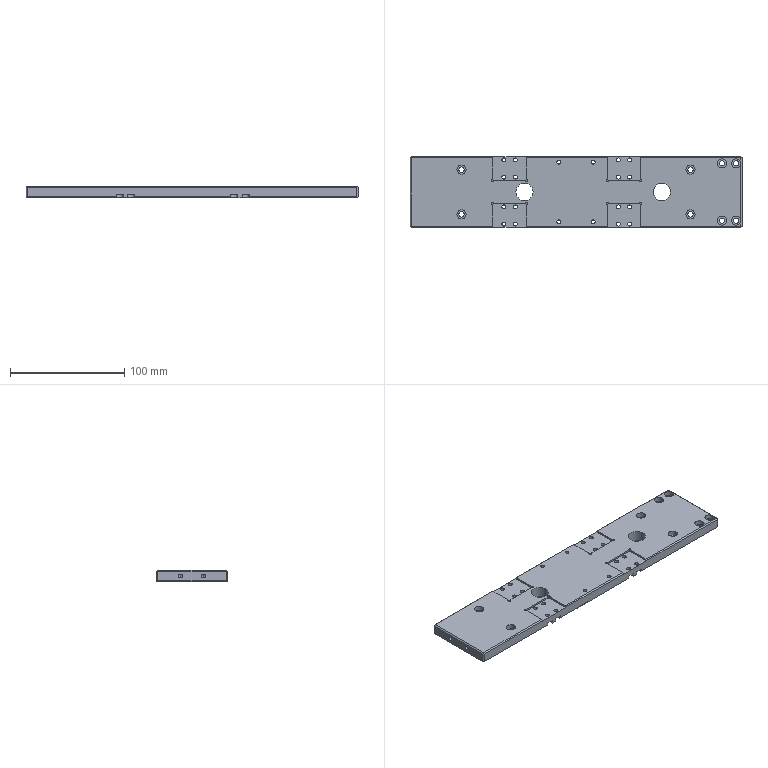Part | STEP file | 01-03 loading sliding base plate | 1 solid | 214 faces | box 290 x 62 x 10 mm | volume 166343 mm3 | cylinder 124 | plane 86 | cone 4 | commonest cylinder face diameters 3.5 x32 6 x24 8 x24 2 x12 3.3 x12 4.5 x8